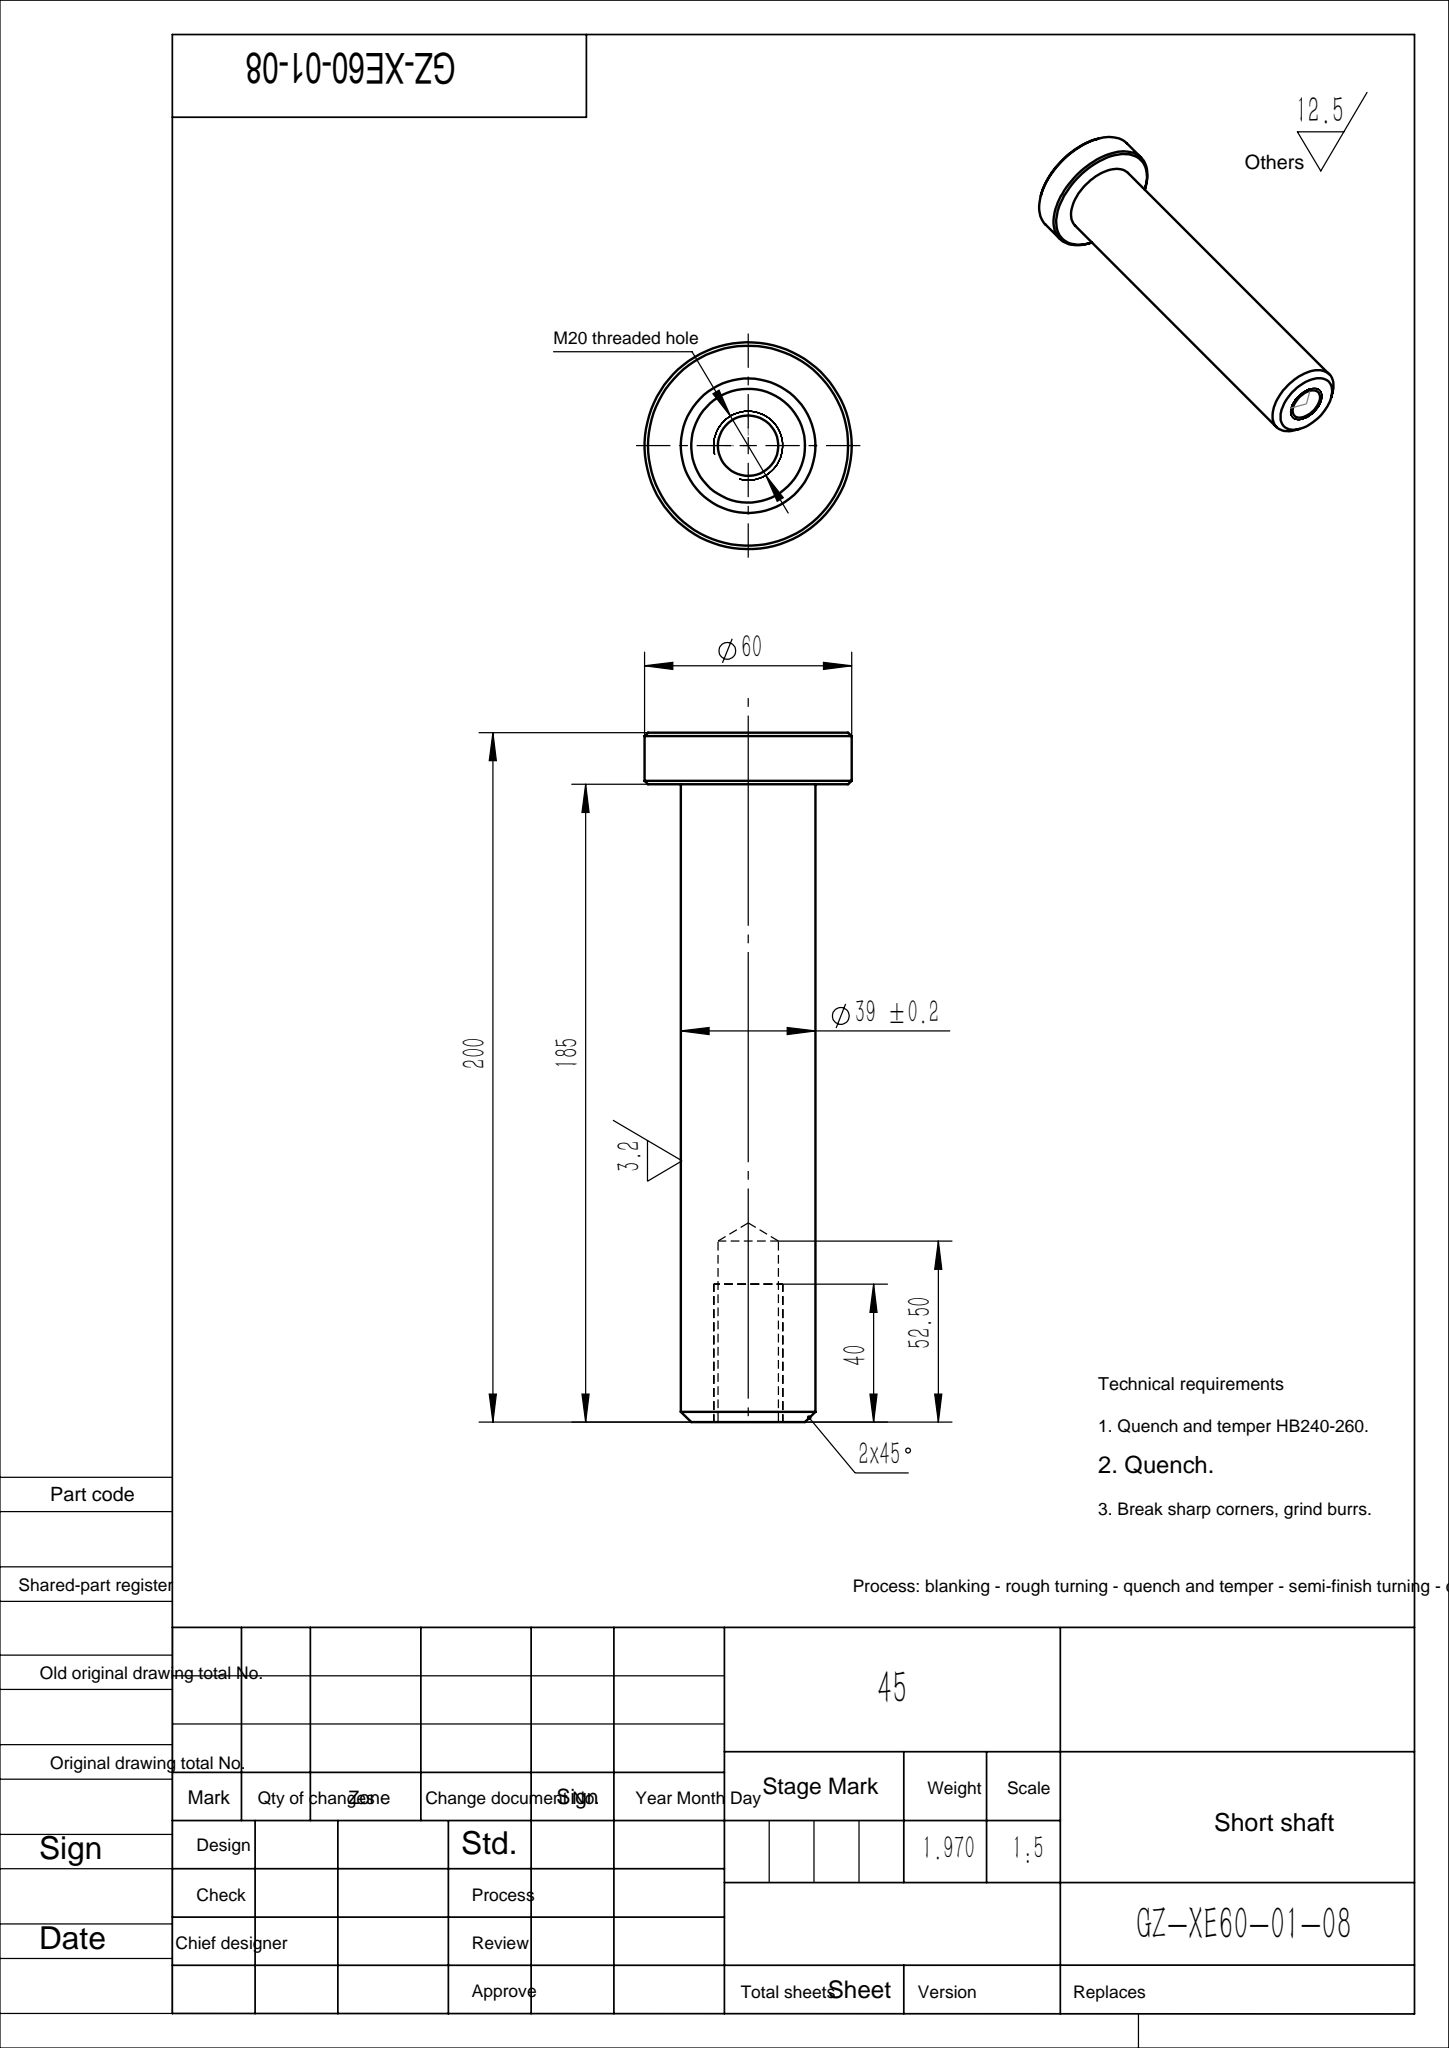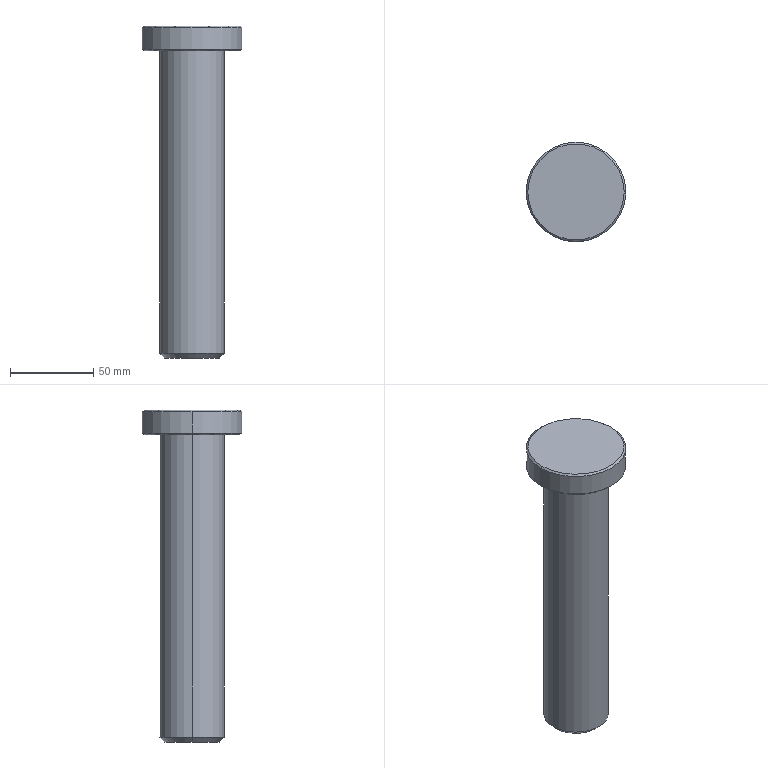Part | SolidWorks | features Chamfer 2, 3DProfileFeature 1, Extrusion 1, HoleWzd 1, ICE 1 | 1 solid | 17 faces | box 60 x 60 x 200 mm | volume 249652 mm3 | cone 8 | cylinder 6 | plane 3 | commonest cylinder face diameters 17.5 x2 39 x2 60 x2
STEP:
#1=CARTESIAN_POINT('',(8.75,0.,52.5));
#2=VERTEX_POINT('',#1);
#3=CARTESIAN_POINT('',(-8.75,0.,52.5));
#4=VERTEX_POINT('',#3);
#5=CARTESIAN_POINT('',(0.,0.,52.5));
#6=DIRECTION('',(0.,0.,-1.));
#7=DIRECTION('',(-1.,0.,0.));
#8=AXIS2_PLACEMENT_3D('',#5,#6,#7);
#9=CIRCLE('',#8,8.75);
#10=EDGE_CURVE('',#2,#4,#9,.T.);
#11=ORIENTED_EDGE('',*,*,#10,.F.);
#12=CARTESIAN_POINT('',(8.75,0.,0.));
#13=VERTEX_POINT('',#12);
#14=CARTESIAN_POINT('',(8.75,0.,0.));
#15=DIRECTION('',(0.,0.,-1.));
#16=VECTOR('',#15,1000.);
#17=LINE('',#14,#16);
#18=EDGE_CURVE('',#2,#13,#17,.T.);
#19=ORIENTED_EDGE('',*,*,#18,.T.);
#20=CARTESIAN_POINT('',(-8.75,0.,0.));
#21=VERTEX_POINT('',#20);
#22=CARTESIAN_POINT('',(0.,0.,0.));
#23=DIRECTION('',(0.,0.,-1.));
#24=DIRECTION('',(-1.,0.,0.));
#25=AXIS2_PLACEMENT_3D('',#22,#23,#24);
#26=CIRCLE('',#25,8.75);
#27=EDGE_CURVE('',#13,#21,#26,.T.);
#28=ORIENTED_EDGE('',*,*,#27,.T.);
#29=CARTESIAN_POINT('',(-8.75,0.,0.));
#30=DIRECTION('',(0.,0.,-1.));
#31=VECTOR('',#30,1000.);
#32=LINE('',#29,#31);
#33=EDGE_CURVE('',#4,#21,#32,.T.);
#34=ORIENTED_EDGE('',*,*,#33,.F.);
#35=EDGE_LOOP('',(#11,#19,#28,#34));
#36=FACE_OUTER_BOUND('',#35,.T.);
#37=CARTESIAN_POINT('',(0.,0.,0.));
#38=DIRECTION('',(0.,0.,-1.));
#39=DIRECTION('',(-1.,0.,0.));
#40=AXIS2_PLACEMENT_3D('',#37,#38,#39);
#41=CYLINDRICAL_SURFACE('',#40,8.75);
#42=ADVANCED_FACE('',(#36),#41,.F.);
#43=CARTESIAN_POINT('',(0.,0.,57.758));
#44=VERTEX_POINT('',#43);
#45=CARTESIAN_POINT('',(-8.75,0.,52.5));
#46=DIRECTION('',(-0.8572,0.,-0.515));
#47=VECTOR('',#46,1000.);
#48=LINE('',#45,#47);
#49=EDGE_CURVE('',#44,#4,#48,.T.);
#50=ORIENTED_EDGE('',*,*,#49,.F.);
#51=CARTESIAN_POINT('',(8.75,0.,52.5));
#52=DIRECTION('',(0.8572,0.,-0.515));
#53=VECTOR('',#52,1000.);
#54=LINE('',#51,#53);
#55=EDGE_CURVE('',#44,#2,#54,.T.);
#56=ORIENTED_EDGE('',*,*,#55,.T.);
#57=ORIENTED_EDGE('',*,*,#10,.T.);
#58=EDGE_LOOP('',(#50,#56,#57));
#59=FACE_OUTER_BOUND('',#58,.T.);
#60=CARTESIAN_POINT('',(0.,0.,52.5));
#61=DIRECTION('',(0.,0.,-1.));
#62=DIRECTION('',(-1.,0.,0.));
#63=AXIS2_PLACEMENT_3D('',#60,#61,#62);
#64=CONICAL_SURFACE('',#63,8.75,1.03);
#65=ADVANCED_FACE('',(#59),#64,.F.);
#66=CARTESIAN_POINT('',(29.,0.,200.));
#67=VERTEX_POINT('',#66);
#68=CARTESIAN_POINT('',(-29.,0.,200.));
#69=VERTEX_POINT('',#68);
#70=CARTESIAN_POINT('',(0.,0.,200.));
#71=DIRECTION('',(0.,0.,1.));
#72=DIRECTION('',(1.,0.,0.));
#73=AXIS2_PLACEMENT_3D('',#70,#71,#72);
#74=CIRCLE('',#73,29.);
#75=EDGE_CURVE('',#67,#69,#74,.T.);
#76=ORIENTED_EDGE('',*,*,#75,.F.);
#77=CARTESIAN_POINT('',(30.,0.,199.));
#78=VERTEX_POINT('',#77);
#79=CARTESIAN_POINT('',(29.,0.,200.));
#80=DIRECTION('',(0.7071,0.,-0.7071));
#81=VECTOR('',#80,1000.);
#82=LINE('',#79,#81);
#83=EDGE_CURVE('',#67,#78,#82,.T.);
#84=ORIENTED_EDGE('',*,*,#83,.T.);
#85=CARTESIAN_POINT('',(-30.,0.,199.));
#86=VERTEX_POINT('',#85);
#87=CARTESIAN_POINT('',(0.,0.,199.));
#88=DIRECTION('',(0.,0.,-1.));
#89=DIRECTION('',(1.,0.,0.));
#90=AXIS2_PLACEMENT_3D('',#87,#88,#89);
#91=CIRCLE('',#90,30.);
#92=EDGE_CURVE('',#86,#78,#91,.T.);
#93=ORIENTED_EDGE('',*,*,#92,.F.);
#94=CARTESIAN_POINT('',(-29.,0.,200.));
#95=DIRECTION('',(-0.7071,0.,-0.7071));
#96=VECTOR('',#95,1000.);
#97=LINE('',#94,#96);
#98=EDGE_CURVE('',#69,#86,#97,.T.);
#99=ORIENTED_EDGE('',*,*,#98,.F.);
#100=EDGE_LOOP('',(#76,#84,#93,#99));
#101=FACE_OUTER_BOUND('',#100,.T.);
#102=CARTESIAN_POINT('',(0.,0.,200.));
#103=DIRECTION('',(0.,0.,-1.));
#104=DIRECTION('',(-1.,0.,0.));
#105=AXIS2_PLACEMENT_3D('',#102,#103,#104);
#106=CONICAL_SURFACE('',#105,29.,0.7854);
#107=ADVANCED_FACE('',(#101),#106,.T.);
#108=CARTESIAN_POINT('',(-29.,0.,185.));
#109=VERTEX_POINT('',#108);
#110=CARTESIAN_POINT('',(29.,0.,185.));
#111=VERTEX_POINT('',#110);
#112=CARTESIAN_POINT('',(0.,0.,185.));
#113=DIRECTION('',(0.,0.,-1.));
#114=DIRECTION('',(1.,0.,0.));
#115=AXIS2_PLACEMENT_3D('',#112,#113,#114);
#116=CIRCLE('',#115,29.);
#117=EDGE_CURVE('',#109,#111,#116,.T.);
#118=ORIENTED_EDGE('',*,*,#117,.F.);
#119=CARTESIAN_POINT('',(-30.,0.,186.));
#120=VERTEX_POINT('',#119);
#121=CARTESIAN_POINT('',(-30.,0.,186.));
#122=DIRECTION('',(-0.7071,0.,0.7071));
#123=VECTOR('',#122,1000.);
#124=LINE('',#121,#123);
#125=EDGE_CURVE('',#109,#120,#124,.T.);
#126=ORIENTED_EDGE('',*,*,#125,.T.);
#127=CARTESIAN_POINT('',(30.,0.,186.));
#128=VERTEX_POINT('',#127);
#129=CARTESIAN_POINT('',(0.,0.,186.));
#130=DIRECTION('',(0.,0.,1.));
#131=DIRECTION('',(1.,0.,0.));
#132=AXIS2_PLACEMENT_3D('',#129,#130,#131);
#133=CIRCLE('',#132,30.);
#134=EDGE_CURVE('',#128,#120,#133,.T.);
#135=ORIENTED_EDGE('',*,*,#134,.F.);
#136=CARTESIAN_POINT('',(30.,0.,186.));
#137=DIRECTION('',(0.7071,0.,0.7071));
#138=VECTOR('',#137,1000.);
#139=LINE('',#136,#138);
#140=EDGE_CURVE('',#111,#128,#139,.T.);
#141=ORIENTED_EDGE('',*,*,#140,.F.);
#142=EDGE_LOOP('',(#118,#126,#135,#141));
#143=FACE_OUTER_BOUND('',#142,.T.);
#144=CARTESIAN_POINT('',(0.,0.,186.));
#145=DIRECTION('',(0.,0.,1.));
#146=DIRECTION('',(1.,0.,0.));
#147=AXIS2_PLACEMENT_3D('',#144,#145,#146);
#148=CONICAL_SURFACE('',#147,30.,0.7854);
#149=ADVANCED_FACE('',(#143),#148,.T.);
#150=CARTESIAN_POINT('',(-16.5,0.,0.));
#151=VERTEX_POINT('',#150);
#152=CARTESIAN_POINT('',(16.5,0.,0.));
#153=VERTEX_POINT('',#152);
#154=CARTESIAN_POINT('',(0.,0.,0.));
#155=DIRECTION('',(0.,0.,-1.));
#156=DIRECTION('',(1.,0.,0.));
#157=AXIS2_PLACEMENT_3D('',#154,#155,#156);
#158=CIRCLE('',#157,16.5);
#159=EDGE_CURVE('',#151,#153,#158,.T.);
#160=ORIENTED_EDGE('',*,*,#159,.F.);
#161=CARTESIAN_POINT('',(-19.5,0.,3.));
#162=VERTEX_POINT('',#161);
#163=CARTESIAN_POINT('',(-19.5,0.,3.));
#164=DIRECTION('',(-0.7071,0.,0.7071));
#165=VECTOR('',#164,1000.);
#166=LINE('',#163,#165);
#167=EDGE_CURVE('',#151,#162,#166,.T.);
#168=ORIENTED_EDGE('',*,*,#167,.T.);
#169=CARTESIAN_POINT('',(19.5,0.,3.));
#170=VERTEX_POINT('',#169);
#171=CARTESIAN_POINT('',(0.,0.,3.));
#172=DIRECTION('',(0.,0.,1.));
#173=DIRECTION('',(1.,0.,0.));
#174=AXIS2_PLACEMENT_3D('',#171,#172,#173);
#175=CIRCLE('',#174,19.5);
#176=EDGE_CURVE('',#170,#162,#175,.T.);
#177=ORIENTED_EDGE('',*,*,#176,.F.);
#178=CARTESIAN_POINT('',(19.5,0.,3.));
#179=DIRECTION('',(0.7071,0.,0.7071));
#180=VECTOR('',#179,1000.);
#181=LINE('',#178,#180);
#182=EDGE_CURVE('',#153,#170,#181,.T.);
#183=ORIENTED_EDGE('',*,*,#182,.F.);
#184=EDGE_LOOP('',(#160,#168,#177,#183));
#185=FACE_OUTER_BOUND('',#184,.T.);
#186=CARTESIAN_POINT('',(0.,0.,3.));
#187=DIRECTION('',(0.,0.,1.));
#188=DIRECTION('',(1.,0.,0.));
#189=AXIS2_PLACEMENT_3D('',#186,#187,#188);
#190=CONICAL_SURFACE('',#189,19.5,0.7854);
#191=ADVANCED_FACE('',(#185),#190,.T.);
#192=ORIENTED_EDGE('',*,*,#92,.T.);
#193=CARTESIAN_POINT('',(30.,0.,200.));
#194=DIRECTION('',(0.,0.,-1.));
#195=VECTOR('',#194,1000.);
#196=LINE('',#193,#195);
#197=EDGE_CURVE('',#78,#128,#196,.T.);
#198=ORIENTED_EDGE('',*,*,#197,.T.);
#199=ORIENTED_EDGE('',*,*,#134,.T.);
#200=CARTESIAN_POINT('',(-30.,0.,200.));
#201=DIRECTION('',(0.,0.,-1.));
#202=VECTOR('',#201,1000.);
#203=LINE('',#200,#202);
#204=EDGE_CURVE('',#86,#120,#203,.T.);
#205=ORIENTED_EDGE('',*,*,#204,.F.);
#206=EDGE_LOOP('',(#192,#198,#199,#205));
#207=FACE_OUTER_BOUND('',#206,.T.);
#208=CARTESIAN_POINT('',(0.,0.,200.));
#209=DIRECTION('',(0.,0.,-1.));
#210=DIRECTION('',(-1.,0.,0.));
#211=AXIS2_PLACEMENT_3D('',#208,#209,#210);
#212=CYLINDRICAL_SURFACE('',#211,30.);
#213=ADVANCED_FACE('',(#207),#212,.T.);
#214=CARTESIAN_POINT('',(19.5,0.,185.));
#215=VERTEX_POINT('',#214);
#216=CARTESIAN_POINT('',(-19.5,0.,185.));
#217=VERTEX_POINT('',#216);
#218=CARTESIAN_POINT('',(0.,0.,185.));
#219=DIRECTION('',(0.,0.,1.));
#220=DIRECTION('',(1.,0.,0.));
#221=AXIS2_PLACEMENT_3D('',#218,#219,#220);
#222=CIRCLE('',#221,19.5);
#223=EDGE_CURVE('',#215,#217,#222,.T.);
#224=ORIENTED_EDGE('',*,*,#223,.F.);
#225=CARTESIAN_POINT('',(19.5,0.,185.));
#226=DIRECTION('',(0.,0.,-1.));
#227=VECTOR('',#226,1000.);
#228=LINE('',#225,#227);
#229=EDGE_CURVE('',#215,#170,#228,.T.);
#230=ORIENTED_EDGE('',*,*,#229,.T.);
#231=ORIENTED_EDGE('',*,*,#176,.T.);
#232=CARTESIAN_POINT('',(-19.5,0.,185.));
#233=DIRECTION('',(0.,0.,-1.));
#234=VECTOR('',#233,1000.);
#235=LINE('',#232,#234);
#236=EDGE_CURVE('',#217,#162,#235,.T.);
#237=ORIENTED_EDGE('',*,*,#236,.F.);
#238=EDGE_LOOP('',(#224,#230,#231,#237));
#239=FACE_OUTER_BOUND('',#238,.T.);
#240=CARTESIAN_POINT('',(0.,0.,185.));
#241=DIRECTION('',(0.,0.,-1.));
#242=DIRECTION('',(-1.,0.,0.));
#243=AXIS2_PLACEMENT_3D('',#240,#241,#242);
#244=CYLINDRICAL_SURFACE('',#243,19.5);
#245=ADVANCED_FACE('',(#239),#244,.T.);
#246=ORIENTED_EDGE('',*,*,#229,.F.);
#247=CARTESIAN_POINT('',(0.,0.,185.));
#248=DIRECTION('',(0.,0.,1.));
#249=DIRECTION('',(1.,0.,0.));
#250=AXIS2_PLACEMENT_3D('',#247,#248,#249);
#251=CIRCLE('',#250,19.5);
#252=EDGE_CURVE('',#217,#215,#251,.T.);
#253=ORIENTED_EDGE('',*,*,#252,.F.);
#254=ORIENTED_EDGE('',*,*,#236,.T.);
#255=CARTESIAN_POINT('',(0.,0.,3.));
#256=DIRECTION('',(0.,0.,1.));
#257=DIRECTION('',(1.,0.,0.));
#258=AXIS2_PLACEMENT_3D('',#255,#256,#257);
#259=CIRCLE('',#258,19.5);
#260=EDGE_CURVE('',#162,#170,#259,.T.);
#261=ORIENTED_EDGE('',*,*,#260,.T.);
#262=EDGE_LOOP('',(#246,#253,#254,#261));
#263=FACE_OUTER_BOUND('',#262,.T.);
#264=CARTESIAN_POINT('',(0.,0.,185.));
#265=DIRECTION('',(0.,0.,-1.));
#266=DIRECTION('',(-1.,0.,0.));
#267=AXIS2_PLACEMENT_3D('',#264,#265,#266);
#268=CYLINDRICAL_SURFACE('',#267,19.5);
#269=ADVANCED_FACE('',(#263),#268,.T.);
#270=CARTESIAN_POINT('',(0.,0.,0.));
#271=DIRECTION('',(0.,0.,-1.));
#272=DIRECTION('',(-1.,0.,0.));
#273=AXIS2_PLACEMENT_3D('',#270,#271,#272);
#274=CIRCLE('',#273,8.75);
#275=EDGE_CURVE('',#21,#13,#274,.T.);
#276=ORIENTED_EDGE('',*,*,#275,.F.);
#277=ORIENTED_EDGE('',*,*,#27,.F.);
#278=EDGE_LOOP('',(#276,#277));
#279=FACE_BOUND('',#278,.T.);
#280=CARTESIAN_POINT('',(0.,0.,0.));
#281=DIRECTION('',(0.,0.,-1.));
#282=DIRECTION('',(1.,0.,0.));
#283=AXIS2_PLACEMENT_3D('',#280,#281,#282);
#284=CIRCLE('',#283,16.5);
#285=EDGE_CURVE('',#153,#151,#284,.T.);
#286=ORIENTED_EDGE('',*,*,#285,.T.);
#287=ORIENTED_EDGE('',*,*,#159,.T.);
#288=EDGE_LOOP('',(#286,#287));
#289=FACE_OUTER_BOUND('',#288,.T.);
#290=CARTESIAN_POINT('',(0.,0.,0.));
#291=DIRECTION('',(0.,0.,1.));
#292=DIRECTION('',(1.,0.,0.));
#293=AXIS2_PLACEMENT_3D('',#290,#291,#292);
#294=PLANE('',#293);
#295=ADVANCED_FACE('',(#279,#289),#294,.F.);
#296=ORIENTED_EDGE('',*,*,#197,.F.);
#297=CARTESIAN_POINT('',(0.,0.,199.));
#298=DIRECTION('',(0.,0.,-1.));
#299=DIRECTION('',(1.,0.,0.));
#300=AXIS2_PLACEMENT_3D('',#297,#298,#299);
#301=CIRCLE('',#300,30.);
#302=EDGE_CURVE('',#78,#86,#301,.T.);
#303=ORIENTED_EDGE('',*,*,#302,.T.);
#304=ORIENTED_EDGE('',*,*,#204,.T.);
#305=CARTESIAN_POINT('',(0.,0.,186.));
#306=DIRECTION('',(0.,0.,1.));
#307=DIRECTION('',(1.,0.,0.));
#308=AXIS2_PLACEMENT_3D('',#305,#306,#307);
#309=CIRCLE('',#308,30.);
#310=EDGE_CURVE('',#120,#128,#309,.T.);
#311=ORIENTED_EDGE('',*,*,#310,.T.);
#312=EDGE_LOOP('',(#296,#303,#304,#311));
#313=FACE_OUTER_BOUND('',#312,.T.);
#314=CARTESIAN_POINT('',(0.,0.,200.));
#315=DIRECTION('',(0.,0.,-1.));
#316=DIRECTION('',(-1.,0.,0.));
#317=AXIS2_PLACEMENT_3D('',#314,#315,#316);
#318=CYLINDRICAL_SURFACE('',#317,30.);
#319=ADVANCED_FACE('',(#313),#318,.T.);
#320=CARTESIAN_POINT('',(0.,0.,200.));
#321=DIRECTION('',(0.,0.,1.));
#322=DIRECTION('',(1.,0.,0.));
#323=AXIS2_PLACEMENT_3D('',#320,#321,#322);
#324=CIRCLE('',#323,29.);
#325=EDGE_CURVE('',#69,#67,#324,.T.);
#326=ORIENTED_EDGE('',*,*,#325,.T.);
#327=ORIENTED_EDGE('',*,*,#75,.T.);
#328=EDGE_LOOP('',(#326,#327));
#329=FACE_OUTER_BOUND('',#328,.T.);
#330=CARTESIAN_POINT('',(0.,0.,200.));
#331=DIRECTION('',(0.,0.,1.));
#332=DIRECTION('',(1.,0.,0.));
#333=AXIS2_PLACEMENT_3D('',#330,#331,#332);
#334=PLANE('',#333);
#335=ADVANCED_FACE('',(#329),#334,.T.);
#336=CARTESIAN_POINT('',(0.,0.,185.));
#337=DIRECTION('',(0.,0.,-1.));
#338=DIRECTION('',(1.,0.,0.));
#339=AXIS2_PLACEMENT_3D('',#336,#337,#338);
#340=CIRCLE('',#339,29.);
#341=EDGE_CURVE('',#111,#109,#340,.T.);
#342=ORIENTED_EDGE('',*,*,#341,.T.);
#343=ORIENTED_EDGE('',*,*,#117,.T.);
#344=EDGE_LOOP('',(#342,#343));
#345=FACE_OUTER_BOUND('',#344,.T.);
#346=ORIENTED_EDGE('',*,*,#252,.T.);
#347=ORIENTED_EDGE('',*,*,#223,.T.);
#348=EDGE_LOOP('',(#346,#347));
#349=FACE_BOUND('',#348,.T.);
#350=CARTESIAN_POINT('',(0.,0.,185.));
#351=DIRECTION('',(0.,0.,1.));
#352=DIRECTION('',(1.,0.,0.));
#353=AXIS2_PLACEMENT_3D('',#350,#351,#352);
#354=PLANE('',#353);
#355=ADVANCED_FACE('',(#345,#349),#354,.F.);
#356=ORIENTED_EDGE('',*,*,#167,.F.);
#357=ORIENTED_EDGE('',*,*,#285,.F.);
#358=ORIENTED_EDGE('',*,*,#182,.T.);
#359=ORIENTED_EDGE('',*,*,#260,.F.);
#360=EDGE_LOOP('',(#356,#357,#358,#359));
#361=FACE_OUTER_BOUND('',#360,.T.);
#362=CARTESIAN_POINT('',(0.,0.,3.));
#363=DIRECTION('',(0.,0.,1.));
#364=DIRECTION('',(1.,0.,0.));
#365=AXIS2_PLACEMENT_3D('',#362,#363,#364);
#366=CONICAL_SURFACE('',#365,19.5,0.7854);
#367=ADVANCED_FACE('',(#361),#366,.T.);
#368=ORIENTED_EDGE('',*,*,#125,.F.);
#369=ORIENTED_EDGE('',*,*,#341,.F.);
#370=ORIENTED_EDGE('',*,*,#140,.T.);
#371=ORIENTED_EDGE('',*,*,#310,.F.);
#372=EDGE_LOOP('',(#368,#369,#370,#371));
#373=FACE_OUTER_BOUND('',#372,.T.);
#374=CARTESIAN_POINT('',(0.,0.,186.));
#375=DIRECTION('',(0.,0.,1.));
#376=DIRECTION('',(1.,0.,0.));
#377=AXIS2_PLACEMENT_3D('',#374,#375,#376);
#378=CONICAL_SURFACE('',#377,30.,0.7854);
#379=ADVANCED_FACE('',(#373),#378,.T.);
#380=ORIENTED_EDGE('',*,*,#83,.F.);
#381=ORIENTED_EDGE('',*,*,#325,.F.);
#382=ORIENTED_EDGE('',*,*,#98,.T.);
#383=ORIENTED_EDGE('',*,*,#302,.F.);
#384=EDGE_LOOP('',(#380,#381,#382,#383));
#385=FACE_OUTER_BOUND('',#384,.T.);
#386=CARTESIAN_POINT('',(0.,0.,200.));
#387=DIRECTION('',(0.,0.,-1.));
#388=DIRECTION('',(-1.,0.,0.));
#389=AXIS2_PLACEMENT_3D('',#386,#387,#388);
#390=CONICAL_SURFACE('',#389,29.,0.7854);
#391=ADVANCED_FACE('',(#385),#390,.T.);
#392=ORIENTED_EDGE('',*,*,#55,.F.);
#393=ORIENTED_EDGE('',*,*,#49,.T.);
#394=CARTESIAN_POINT('',(0.,0.,52.5));
#395=DIRECTION('',(0.,0.,-1.));
#396=DIRECTION('',(-1.,0.,0.));
#397=AXIS2_PLACEMENT_3D('',#394,#395,#396);
#398=CIRCLE('',#397,8.75);
#399=EDGE_CURVE('',#4,#2,#398,.T.);
#400=ORIENTED_EDGE('',*,*,#399,.T.);
#401=EDGE_LOOP('',(#392,#393,#400));
#402=FACE_OUTER_BOUND('',#401,.T.);
#403=CARTESIAN_POINT('',(0.,0.,52.5));
#404=DIRECTION('',(0.,0.,-1.));
#405=DIRECTION('',(-1.,0.,0.));
#406=AXIS2_PLACEMENT_3D('',#403,#404,#405);
#407=CONICAL_SURFACE('',#406,8.75,1.03);
#408=ADVANCED_FACE('',(#402),#407,.F.);
#409=ORIENTED_EDGE('',*,*,#18,.F.);
#410=ORIENTED_EDGE('',*,*,#399,.F.);
#411=ORIENTED_EDGE('',*,*,#33,.T.);
#412=ORIENTED_EDGE('',*,*,#275,.T.);
#413=EDGE_LOOP('',(#409,#410,#411,#412));
#414=FACE_OUTER_BOUND('',#413,.T.);
#415=CARTESIAN_POINT('',(0.,0.,0.));
#416=DIRECTION('',(0.,0.,-1.));
#417=DIRECTION('',(-1.,0.,0.));
#418=AXIS2_PLACEMENT_3D('',#415,#416,#417);
#419=CYLINDRICAL_SURFACE('',#418,8.75);
#420=ADVANCED_FACE('',(#414),#419,.F.);
#421=CLOSED_SHELL('',(#42,#65,#107,#149,#191,#213,#245,#269,#295,#319,#335,#355,#367,#379,#391,#408,#420));
#422=MANIFOLD_SOLID_BREP('',#421);
#423=CARTESIAN_POINT('',(0.,0.,0.));
#424=DIRECTION('',(0.,0.,1.));
#425=DIRECTION('',(1.,0.,0.));
#426=AXIS2_PLACEMENT_3D('',#423,#424,#425);
#427=(LENGTH_UNIT()NAMED_UNIT(*)SI_UNIT(.MILLI.,.METRE.));
#428=UNCERTAINTY_MEASURE_WITH_UNIT(LENGTH_MEASURE(0.00001),#427,'','');
#429=(NAMED_UNIT(*)PLANE_ANGLE_UNIT()SI_UNIT($,.RADIAN.));
#430=(NAMED_UNIT(*)SI_UNIT($,.STERADIAN.)SOLID_ANGLE_UNIT());
#431=(GEOMETRIC_REPRESENTATION_CONTEXT(3)GLOBAL_UNCERTAINTY_ASSIGNED_CONTEXT((#428))GLOBAL_UNIT_ASSIGNED_CONTEXT((#427,#429,#430))REPRESENTATION_CONTEXT('',''));
#432=ADVANCED_BREP_SHAPE_REPRESENTATION('',(#422,#426),#431);